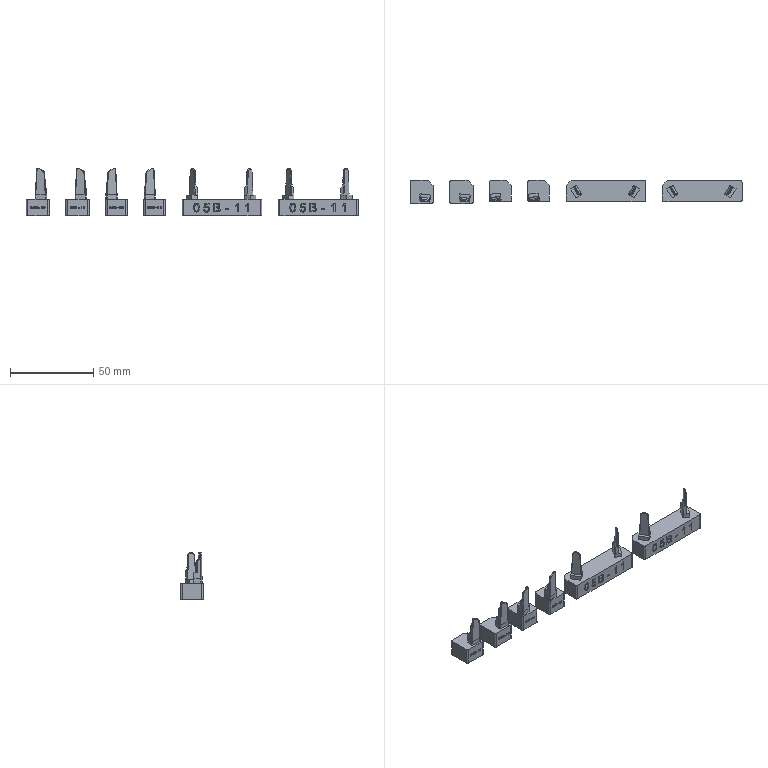NC program | NX | posted with a generic post | part box 200 x 14 x 28.763 mm
Lines 1 to 971 of 209396:
N10 G17 G21 G94 G90
(CAVITY_MILL_C_0_0 , TOOL : D8-0.075)
N12 T00 M6
N14 G53
N16 G17 G0 G90 X0. Y-20.632 S10000 M3
N18 G43 Z30.1 H0
N20 Z0.303
N22 Z-0.197
N24 Y-12.39
N26 G94 G1 X-101.064 F4500.
N28 G2 X-105.391 Y-7.996 R4.39
N30 G1 Y7.992
N32 G2 X-101.065 Y12.388 R4.386
N34 G1 X101.064
N36 G2 X105.391 Y8.077 R4.388
N38 G1 Y-7.992
N40 G2 X101.064 Y-12.39 R4.388
N42 G1 X0.
N44 Y-6.895
N46 X-18.587
N48 G3 X-18.103 Y-3.95 R5.547
N50 G1 X-18.136 Y-3.678
N52 G3 X-22.479 Y1.041 R5.548
N54 X-26.529 Y0.598 R6.416
N56 X-29.797 Y-4.389 R5.567
N58 X-29.293 Y-6.895 R5.637
N60 G1 X-28.292 Y-6.439
N62 G2 X-28.698 Y-4.414 R4.538
N64 X-26.072 Y-0.401 R4.468
N66 X-22.711 Y-0.033 R5.317
N68 X-19.226 Y-3.818 R4.449
N70 G1 X-19.196 Y-4.071
N72 G2 X-21.423 Y-8.426 R4.448
N74 X-25.955 Y-8.728 R5.225
N76 X-28.292 Y-6.439 R4.538
N78 G1 X-29.293 Y-6.895
N80 X-41.584
N82 G3 X-41.105 Y-3.94 R5.551
N84 G1 X-41.135 Y-3.688
N86 G3 X-45.119 Y0.954 R5.558
N88 X-49.527 Y0.603 R6.444
N90 X-52.771 Y-4.882 R5.552
N92 X-52.293 Y-6.895 R5.545
N94 G1 X-51.29 Y-6.446
N96 G2 X-51.674 Y-4.815 R4.446
N98 X-49.071 Y-0.397 R4.453
N100 X-45.422 Y-0.103 R5.345
N102 X-42.226 Y-3.818 R4.459
N104 G1 X-42.196 Y-4.071
N106 G2 X-44.61 Y-8.533 R4.452
N108 X-48.26 Y-8.955 R5.307
N110 X-51.29 Y-6.446 R4.446
N112 G1 X-52.293 Y-6.895
N114 X-63.012
N116 G3 X-62.76 Y-5.757 R5.533
N118 X-65.574 Y-0.105 R5.554
N120 X-70.474 Y0.422 R6.372
N122 X-74.365 Y-4.188 R5.543
N124 G1 X-74.395 Y-4.44
N126 G3 X-74.118 Y-6.895 R5.546
N128 G1 X-73.08 Y-6.531
N130 G2 X-73.304 Y-4.571 R4.447
N132 G1 X-73.274 Y-4.318
N134 G2 X-70.16 Y-0.631 R4.444
N136 X-66.105 Y-1.067 R5.273
N138 X-63.85 Y-5.617 R4.455
N140 X-66.916 Y-9.362 R4.434
N142 X-71.377 Y-8.742 R5.232
N144 X-73.08 Y-6.531 R4.447
N146 G1 X-74.118 Y-6.895
N148 X-87.012
N150 G3 X-86.76 Y-5.757 R5.542
N152 X-89.482 Y-0.152 R5.565
N154 X-94.383 Y0.453 R6.419
N156 X-98.365 Y-4.188 R5.558
N158 G1 X-98.395 Y-4.44
N160 G3 X-98.119 Y-6.895 R5.541
N162 G1 X-97.082 Y-6.531
N164 G2 X-97.304 Y-4.571 R4.442
N166 G1 X-97.274 Y-4.318
N168 G2 X-94.087 Y-0.606 R4.459
N170 X-90.032 Y-1.104 R5.32
N172 X-87.85 Y-5.617 R4.466
N174 X-90.843 Y-9.341 R4.443
N176 X-95.248 Y-8.827 R5.257
N178 X-97.082 Y-6.531 R4.442
N180 G1 X-98.119 Y-6.895
N182 X-99.896
N184 Y6.893
N186 X-77.943
N188 Y1.398
N190 G3 X-79.34 Y-1.4 R11.038
N192 G1 X-81.8
N194 G3 X-83.225 Y1.398 R11.06
N196 G1 X-86.922 Y2.926
N198 X-83.225 Y1.398
N200 X-77.943
N202 X-74.269 Y2.935
N204 X-77.943 Y1.398
N206 Y6.893
N208 X-56.605
N210 Y1.398
N212 G3 X-57.828 Y-1.319 R11.047
N214 X-59.226 Y1.398 R11.049
N216 G1 X-62.925 Y2.925
N218 X-59.226 Y1.398
N220 X-56.605
N222 Y6.893
N224 X-33.606
N226 Y1.398
N228 G3 X-34.857 Y-1.4 R11.062
N230 G1 X-36.007
N232 G3 X-37.232 Y1.398 R11.053
N234 G1 X-33.606
N236 Y6.893
N238 X99.896
N240 Y-6.895
N242 X0.
N244 Y-1.4
N246 X-13.007
N248 G3 X-14.231 Y1.398 R11.043
N250 G1 X94.401
N252 Y-1.4
N254 X0.
N256 Z2.803
N258 G0 Z30.1
N260 Y-20.632
N262 Z0.006
N264 Z-0.494
N266 Y-12.39
N268 G1 X-101.064
N270 G2 X-105.391 Y-7.996 R4.39
N272 G1 Y7.992
N274 G2 X-101.065 Y12.388 R4.386
N276 G1 X101.064
N278 G2 X105.391 Y8.077 R4.388
N280 G1 Y-7.992
N282 G2 X101.064 Y-12.39 R4.388
N284 G1 X0.
N286 Y-6.895
N288 X-18.292
N290 G3 X-17.815 Y-3.908 R5.618
N292 G1 X-17.847 Y-3.642
N294 G3 X-19.013 Y-0.856 R5.512
N296 X-23.738 Y1.279 R5.697
N298 X-24.88 Y1.167 R11.408
N300 X-26.932 Y0.599 R6.733
N302 X-29.794 Y-6.895 R5.693
N304 G1 X-28.789 Y-6.45
N306 G2 X-26.477 Y-0.401 R4.594
N308 X-24.739 Y0.076 R5.634
N310 X-23.685 Y0.181 R10.309
N312 X-19.872 Y-1.542 R4.598
N314 X-18.938 Y-3.772 R4.413
N316 G1 X-18.907 Y-4.038
N318 G2 X-21.074 Y-8.425 R4.519
N320 X-22.85 Y-9.057 R4.782
N322 G1 X-23.116 Y-9.095
N324 G2 X-24.333 Y-9.198 R10.067
N326 X-27.115 Y-8.426 R5.017
N328 X-28.789 Y-6.45 R4.594
N330 G1 X-29.794 Y-6.895
N332 X-41.291
N334 G3 X-40.815 Y-3.908 R5.618
N336 G1 X-40.846 Y-3.651
N338 G3 X-42.925 Y0.058 R5.62
N340 X-46.885 Y1.273 R5.755
N342 X-48.197 Y1.121 R14.817
N344 X-49.935 Y0.598 R6.858
N346 X-52.793 Y-6.895 R5.694
N348 G1 X-51.789 Y-6.45
N350 G2 X-49.482 Y-0.403 R4.595
N352 X-48.023 Y0.036 R5.759
N354 X-46.808 Y0.176 R13.718
N356 X-43.609 Y-0.802 R4.656
N358 X-41.937 Y-3.782 R4.521
N360 G1 X-41.907 Y-4.038
N362 G2 X-44.61 Y-8.702 R4.519
N364 X-46.233 Y-9.108 R5.121
N366 X-47.449 Y-9.2 R8.406
N368 X-50.115 Y-8.426 R5.025
N370 X-51.789 Y-6.45 R4.595
N372 G1 X-52.793 Y-6.895
N374 X-62.514
N376 G3 X-62.951 Y-2.272 R5.744
N378 X-66.544 Y0.459 R5.994
N380 X-67.993 Y0.714 R9.285
N382 X-70.92 Y0.464 R6.098
N384 X-74.654 Y-4.151 R5.602
N386 G1 X-74.685 Y-4.408
N388 G3 X-74.411 Y-6.895 R5.601
N390 G1 X-73.373 Y-6.534
N392 G2 X-73.593 Y-4.538 R4.502
N394 G1 X-73.563 Y-4.282
N396 G2 X-70.566 Y-0.576 R4.503
N398 X-68.132 Y-0.377 R4.999
N400 X-66.831 Y-0.602 R8.186
N402 X-63.91 Y-2.809 R4.895
N404 X-64.744 Y-8.426 R4.645
N406 X-68.132 Y-9.699 R4.948
N408 X-69.349 Y-9.599 R9.552
N410 X-72.105 Y-8.426 R4.809
N412 X-73.373 Y-6.534 R4.502
N414 G1 X-74.411 Y-6.895
N416 X-86.514
N418 G3 X-87.276 Y-1.771 R5.713
N420 X-91.051 Y0.575 R6.069
N422 X-92.353 Y0.756 R17.879
N424 X-94.334 Y0.634 R6.031
N426 X-98.654 Y-4.151 R5.614
N428 G1 X-98.685 Y-4.408
N430 G3 X-98.411 Y-6.895 R5.607
N432 G1 X-97.373 Y-6.534
N434 G2 X-97.593 Y-4.538 R4.508
N436 G1 X-97.563 Y-4.282
N438 G2 X-94.087 Y-0.437 R4.515
N440 X-92.465 Y-0.337 R4.932
N442 X-91.249 Y-0.506 R16.78
N444 X-88.171 Y-2.407 R4.97
N446 X-89.239 Y-8.827 R4.614
N448 X-92.06 Y-9.7 R5.
N450 X-93.276 Y-9.607 R8.43
N452 X-96.115 Y-8.418 R4.867
N454 X-97.373 Y-6.534 R4.508
N456 G1 X-98.411 Y-6.895
N458 X-99.896
N460 Y6.893
N462 X-78.276
N464 Y1.398
N466 G3 X-79.646 Y-1.4 R11.097
N468 G1 X-81.346
N470 G3 X-82.787 Y1.398 R11.208
N472 G1 X-86.501 Y2.918
N474 X-82.787 Y1.398
N476 X-78.276
N478 X-74.632 Y2.947
N480 X-78.276 Y1.398
N482 Y6.893
N484 X-57.039
N486 Y1.398
N488 G3 X-57.86 Y-0.155 R11.189
N490 X-58.157 Y0.413 R11.239
N492 G1 X-58.19 Y0.471
N494 X-58.224 Y0.529
N496 G3 X-58.793 Y1.398 R11.489
N498 G1 X-62.504 Y2.919
N500 X-58.793 Y1.398
N502 X-57.039
N504 Y6.893
N506 X-34.039
N508 Y1.398
N510 G3 X-35.312 Y-1.4 R11.188
N512 G1 X-35.705
N514 G3 X-36.905 Y1.398 R11.115
N516 G1 X-34.039
N518 Y6.893
N520 X-0.953
N522 G3 X-5.721 Y0.969 R5.608
N524 X-5.13 Y-1.277 R6.159
N526 X-3.005 Y-4.222 R11.117
N528 X3.899 Y-4.835 R5.553
N530 X6.261 Y1.057 R5.502
N532 X5.428 Y3.12 R7.766
N534 X3.776 Y5.375 R8.315
N536 X0.701 Y6.893 R5.608
N538 G1 X0.539 Y5.806
N540 G2 X3.011 Y4.585 R4.509
N542 X4.461 Y2.597 R7.216
N544 X5.192 Y0.802 R6.667
N546 X3.312 Y-3.907 R4.403
N548 G1 X3.139 Y-4.016
N550 G2 X-2.231 Y-3.442 R4.454
N552 X-4.139 Y-0.802 R10.018
N554 X-4.625 Y1.043 R5.06
N556 X0.539 Y5.806 R4.509
N558 G1 X0.701 Y6.893
N560 X34.344
N562 G3 X31.79 Y5.848 R5.613
N564 X30.245 Y4.232 R6.854
N566 X28.879 Y1.58 R11.86
N568 X31.274 Y-4.945 R5.541
N570 X38.088 Y-4.142 R5.531
N572 X39.321 Y-2.643 R10.808
N574 X40.559 Y-0.086 R7.654
N576 X38.27 Y5.987 R5.613
N578 X35.914 Y6.893 R5.613
N580 G1 X35.761 Y5.805
N582 G2 X39.498 Y0.201 R4.514
N584 X38.425 Y-2.006 R6.555
N586 X37.311 Y-3.366 R9.709
N588 X31.861 Y-4.016 R4.432
N590 G1 X31.688 Y-3.907
N592 G2 X29.912 Y1.204 R4.442
N594 X31.151 Y3.611 R10.761
N596 X32.444 Y4.964 R5.755
N598 X35.761 Y5.805 R4.514
N600 G1 X35.914 Y6.893
N602 X57.08
N604 G3 X52.383 Y0.173 R5.613
N606 X53.437 Y-2.287 R7.253
N608 G1 X53.668 Y-2.625
N610 G3 X54.989 Y-4.217 R10.717
N612 X61.899 Y-4.835 R5.555
N614 X64.261 Y1.057 R5.504
N616 X63.423 Y3.132 R8.006
N618 X61.736 Y5.41 R8.242
N620 X58.668 Y6.893 R5.613
N622 G1 X58.513 Y5.805
N624 G2 X60.978 Y4.614 R4.514
N626 X62.455 Y2.61 R7.143
N628 X63.192 Y0.802 R6.907
N630 X61.312 Y-3.907 R4.405
N632 G1 X61.139 Y-4.016
N634 G2 X55.763 Y-3.437 R4.456
N636 X54.576 Y-2.006 R9.618
N638 G1 X54.344 Y-1.666
N640 G2 X53.459 Y0.401 R6.154
N642 X58.513 Y5.805 R4.514
N644 G1 X58.668 Y6.893
N646 X92.339
N648 G3 X89.551 Y5.662 R5.613
N650 X88.246 Y4.233 R6.999
N652 X86.88 Y1.579 R11.824
N654 X89.274 Y-4.945 R5.532
N656 X96.14 Y-4.091 R5.534
N658 X97.879 Y-1.767 R12.049
N660 X98.606 Y0.111 R7.004
N662 X96.059 Y6.123 R5.613
N664 X93.916 Y6.893 R5.613
N666 G1 X93.762 Y5.805
N668 G2 X97.535 Y0.357 R4.514
N670 X96.926 Y-1.219 R5.905
N672 X95.353 Y-3.325 R10.95
N674 X89.861 Y-4.016 R4.435
N676 G1 X89.688 Y-3.907
N678 G2 X87.913 Y1.204 R4.433
N680 X89.152 Y3.611 R10.725
N682 X90.252 Y4.815 R5.9
N684 X93.762 Y5.805 R4.514
N686 G1 X93.916 Y6.893
N688 X99.896
N690 Y-6.895
N692 X69.841
N694 Y-1.4
N696 G3 X69.786 Y1.398 R10.999
N698 G1 X81.208
N700 G3 X81.157 Y-1.4 R11.027
N702 G1 X69.841
N704 Y-6.895
N706 X45.895
N708 Y-1.4
N710 G3 X46.237 Y1.398 R11.108
N712 G1 X46.767
N714 G3 X47.014 Y-0.993 R11.108
N716 X47.11 Y-1.4 R12.748
N718 G1 X45.895
N720 Y-6.895
N722 X11.842
N724 Y-1.4
N726 G3 X11.787 Y1.398 R10.997
N728 G1 X23.208
N730 G3 X23.158 Y-1.4 R11.036
N732 G1 X11.842
N734 Y-6.895
N736 X0.
N738 X-10.893 Y-1.4
N740 X-12.701
N742 G3 X-13.901 Y1.398 R11.007
N744 G1 X-11.229
N746 G3 X-11.204 Y0.599 R11.103
N748 X-10.893 Y-1.4 R11.654
N750 G1 Z2.506
N752 G0 X0. Y-20.632
N754 Z-0.29
N756 Z-0.79
N758 Y-12.39
N760 G1 X-101.064
N762 G2 X-105.391 Y-7.996 R4.39
N764 G1 Y7.992
N766 G2 X-101.065 Y12.388 R4.386
N768 G1 X101.064
N770 G2 X105.391 Y8.077 R4.388
N772 G1 Y-7.992
N774 G2 X101.064 Y-12.39 R4.388
N776 G1 X0.
N778 Y-6.895
N780 X-18.153
N782 G3 X-17.677 Y-3.893 R5.641
N784 G1 X-17.708 Y-3.633
N786 G3 X-23.575 Y1.314 R5.634
N788 X-24.13 Y1.264 R7.606
N790 G1 X-25.506 Y1.09
N792 G3 X-27.673 Y0.411 R6.566
N794 X-30.698 Y-5.35 R5.609
N796 X-30.298 Y-6.895 R5.534
N798 G1 X-29.285 Y-6.469
N800 G2 X-29.607 Y-5.216 R4.435
N802 X-27.172 Y-0.568 R4.51
N804 X-25.368 Y0. R5.467
N806 G1 X-23.992 Y0.174
N808 G2 X-23.522 Y0.216 R6.507
N810 X-18.8 Y-3.764 R4.535
N812 G1 X-18.769 Y-4.023
N814 G2 X-22.711 Y-9.051 R4.542
N816 G1 X-24.333 Y-9.235
N818 G2 X-27.172 Y-8.72 R5.18
N820 X-29.285 Y-6.469 R4.435
N822 G1 X-30.298 Y-6.895
N824 X-41.152
N826 G3 X-40.677 Y-3.893 R5.639
N828 G1 X-40.708 Y-3.633
N830 G3 X-46.742 Y1.303 R5.636
N832 X-46.991 Y1.276 R9.11
N834 G1 X-48.499 Y1.091
N836 G3 X-51.165 Y0.125 R6.488
N838 X-53.698 Y-5.352 R5.571
N840 X-53.299 Y-6.895 R5.527
N842 G1 X-52.286 Y-6.469
N844 G2 X-52.607 Y-5.216 R4.428
N846 X-50.575 Y-0.802 R4.472
N848 X-48.365 Y0. R5.389
N850 G1 X-46.856 Y0.185
N852 G2 X-46.638 Y0.209 R8.011
N854 X-41.8 Y-3.764 R4.537
N856 G1 X-41.769 Y-4.023
N858 G2 X-45.422 Y-9.004 R4.54
N860 X-47.449 Y-9.245 R34.868
N862 X-50.288 Y-8.661 R5.185
N864 X-52.286 Y-6.469 R4.428
N866 G1 X-53.299 Y-6.895
N868 X-62.02
N870 G3 X-61.856 Y-6.227 R5.565
N872 X-63.819 Y-0.751 R5.598
N874 X-66.738 Y0.548 R6.312
N876 X-68.838 Y0.809 R39.164
N878 G1 X-68.882 Y0.812
N880 G3 X-74.792 Y-4.133 R5.636
N882 G1 X-74.823 Y-4.393
N884 G3 X-74.55 Y-6.895 R5.638
N886 G1 X-73.511 Y-6.535
N888 G2 X-73.731 Y-4.523 R4.539
N890 G1 X-73.7 Y-4.264
N892 G2 X-68.943 Y-0.285 R4.537
N894 X-66.916 Y-0.536 R38.065
N896 X-64.51 Y-1.605 R5.213
N898 X-62.935 Y-6.019 R4.499
N900 X-65.698 Y-9.39 R4.466
N902 X-68.248 Y-9.725 R5.334
N904 G1 X-69.754 Y-9.555
N906 G2 X-73.511 Y-6.535 R4.539
N908 G1 X-74.55 Y-6.895
N910 X-86.019
N912 G3 X-85.855 Y-6.226 R5.537
N914 X-87.818 Y-0.751 R5.602
N916 X-90.847 Y0.565 R6.297
N918 X-92.757 Y0.804 R47.498
N920 X-98.792 Y-4.133 R5.638
N922 G1 X-98.823 Y-4.393
N924 G3 X-98.548 Y-6.895 R5.641
N926 G1 X-97.51 Y-6.534
N928 G2 X-97.731 Y-4.523 R4.542
N930 G1 X-97.7 Y-4.264
N932 G2 X-92.871 Y-0.29 R4.539
N934 X-91.006 Y-0.523 R46.399
N936 X-88.51 Y-1.605 R5.198
N938 X-86.935 Y-6.019 R4.503
N940 X-89.221 Y-9.165 R4.438
N942 X-92.06 Y-9.744 R5.186
N944 G1 X-93.682 Y-9.563
N946 G2 X-97.51 Y-6.534 R4.542
N948 G1 X-98.548 Y-6.895
N950 X-99.896
N952 Y6.893
N954 X-78.432
N956 Y1.398
N958 G3 X-79.791 Y-1.4 R11.131
N960 G1 X-80.884
N962 G3 X-82.352 Y1.398 R11.097
N964 G1 X-86.084 Y2.911
N966 X-82.352 Y1.398
N968 X-78.432
N970 X-74.8 Y2.953
N972 X-78.432 Y1.398
N974 Y6.893
N976 X-57.493
N978 Y1.398
N980 G3 X-57.896 Y0.718 R11.066
N982 X-58.351 Y1.398 R11.093
N984 G1 X-62.084 Y2.911
N986 X-58.351 Y1.398
N988 X-57.493
N990 Y6.893
N992 X-34.488
N994 Y1.398
N996 G3 X-35.662 Y-1.047 R11.104
N998 X-36.75 Y1.398 R11.131
N1000 G1 X-34.488
N1002 Y6.893
N1004 X-2.496
N1006 G3 X-3.264 Y6.493 R5.575
N1008 G1 X-3.448 Y6.377
N1010 G3 X-5.955 Y2.474 R5.548
N1012 X-5.186 Y-1.363 R6.003
N1014 G1 X-5.001 Y-1.675
N1016 X-4.983 Y-1.704
N1018 X-3.969 Y-3.3
N1020 X-3.951 Y-3.328
N1022 X-3.748 Y-3.627
N1024 G3 X-2.274 Y-5.135 R6.432
N1026 X4.008 Y-5.395 R5.599
N1028 G1 X4.186 Y-5.283
N1030 G3 X6.737 Y-0.351 R5.554
N1032 X5.803 Y2.66 R6.378
N1034 G1 X5.606 Y2.982
N1036 X5.597 Y2.996
N1038 X4.58 Y4.601
N1040 G3 X2.524 Y6.565 R6.177
N1042 X1.874 Y6.893 R5.575
N1044 G1 X1.443 Y5.882
N1046 G2 X1.967 Y5.617 R4.476
N1048 X3.652 Y4.012 R5.078
N1050 G1 X4.669 Y2.407
N1052 X4.867 Y2.085
N1054 G2 X5.639 Y-0.401 R5.279
N1056 X3.598 Y-4.354 R4.455
N1058 G1 X3.42 Y-4.467
N1060 G2 X-1.622 Y-4.25 R4.5
N1062 X-2.839 Y-3.009 R5.333
N1064 G1 X-3.042 Y-2.711
N1066 X-4.055 Y-1.114
N1068 X-4.241 Y-0.802
N1070 G2 X-4.867 Y2.321 R4.904
N1072 X-2.86 Y5.448 R4.449
N1074 G1 X-2.676 Y5.564
N1076 G2 X1.443 Y5.882 R4.476
N1078 G1 X1.874 Y6.893
N1080 X33.121
N1082 G3 X32.469 Y6.564 R5.587
N1084 X30.425 Y4.61 R6.272
N1086 G1 X30.305 Y4.425
N1088 X30.298 Y4.414
N1090 X29.284 Y2.806
N1092 X29.269 Y2.782
N1094 X29.142 Y2.568
N1096 G3 X28.264 Y-0.345 R6.367
N1098 X30.814 Y-5.283 R5.565
N1100 G1 X30.992 Y-5.395
N1102 G3 X37.125 Y-5.241 R5.597
N1104 X38.904 Y-3.399 R6.746
N1106 G1 X39.926 Y-1.794
N1108 X39.939 Y-1.773
N1110 X40.107 Y-1.495
N1112 G3 X40.918 Y0.621 R6.368
N1114 X38.448 Y6.377 R5.607
N1116 G1 X38.264 Y6.493
N1118 G3 X37.494 Y6.893 R5.587
N1120 G1 X37.064 Y5.882
N1122 G2 X37.676 Y5.564 R4.488
N1124 G1 X37.86 Y5.448
N1126 G2 X39.839 Y0.825 R4.508
N1128 X39.168 Y-0.925 R5.269
N1130 G1 X38.999 Y-1.204
N1132 X37.977 Y-2.809
N1134 G2 X36.499 Y-4.337 R5.647
N1136 X31.58 Y-4.467 R4.498
N1138 G1 X31.402 Y-4.354
N1140 G2 X29.361 Y-0.401 R4.466
N1142 X30.086 Y2.006 R5.268
N1144 G1 X30.213 Y2.22
N1146 X31.227 Y3.827
N1148 X31.347 Y4.012
N1150 G2 X33.027 Y5.617 R5.173
N1152 X37.064 Y5.882 R4.488
N1154 G1 X37.494 Y6.893
N1156 X55.508
N1158 G3 X54.736 Y6.493 R5.61
N1160 G1 X54.552 Y6.377
N1162 G3 X52.037 Y2.408 R5.546
N1164 X52.814 Y-1.356 R5.967
N1166 G1 X52.987 Y-1.654
N1168 X53.011 Y-1.694
N1170 X54.096 Y-3.399
N1172 X54.123 Y-3.44
N1174 X54.253 Y-3.624
N1176 G3 X55.718 Y-5.13 R6.357
N1178 X62.008 Y-5.395 R5.597
N1180 G1 X62.186 Y-5.283
N1182 G3 X64.737 Y-0.351 R5.557
N1184 X63.862 Y2.561 R6.382
N1186 G1 X63.81 Y2.65
N1188 X63.789 Y2.685
N1190 X62.629 Y4.521
N1192 G3 X61.223 Y6.089 R6.327
N1194 G1 X61.112 Y6.178
N1196 G3 X59.885 Y6.893 R5.61
N1198 G1 X59.457 Y5.881
N1200 G2 X60.427 Y5.319 R4.511
N1202 G1 X60.538 Y5.23
N1204 G2 X61.7 Y3.934 R5.228
N1206 G1 X62.86 Y2.098
N1208 X62.913 Y2.006
N1210 G2 X63.639 Y-0.401 R5.283
N1212 X61.598 Y-4.354 R4.458
N1214 G1 X61.42 Y-4.467
N1216 G2 X56.371 Y-4.246 R4.498
N1218 X55.155 Y-2.996 R5.258
N1220 G1 X55.023 Y-2.809
N1222 X53.938 Y-1.104
N1224 X53.764 Y-0.802
N1226 G2 X53.127 Y2.268 R4.868
N1228 X55.14 Y5.448 R4.447
N1230 G1 X55.324 Y5.564
N1232 G2 X59.457 Y5.881 R4.511
N1234 G1 X59.885 Y6.893
N1236 X91.121
N1238 G3 X90.468 Y6.564 R5.589
N1240 X88.419 Y4.6 R6.285
N1242 G1 X87.402 Y2.995
N1244 X87.389 Y2.974
N1246 X87.148 Y2.573
N1248 G3 X86.264 Y-0.347 R6.293
N1250 X88.807 Y-5.278 R5.563
N1252 G1 X89.003 Y-5.402
N1254 G3 X95.117 Y-5.246 R5.596
N1256 X96.904 Y-3.399 R6.706
N1258 G1 X97.926 Y-1.794
N1260 X97.937 Y-1.776
N1262 X98.182 Y-1.374
N1264 G3 X99.012 Y1.582 R6.14
N1266 X96.448 Y6.377 R5.58
N1268 G1 X96.264 Y6.493
N1270 G3 X95.494 Y6.893 R5.589
N1272 G1 X95.064 Y5.882
N1274 G2 X95.676 Y5.564 R4.49
N1276 G1 X95.86 Y5.448
N1278 G2 X97.913 Y1.605 R4.481
N1280 X97.243 Y-0.802 R5.041
N1282 G1 X96.999 Y-1.204
N1284 X95.977 Y-2.809
N1286 G2 X94.493 Y-4.341 R5.607
N1288 X89.58 Y-4.467 R4.497
N1290 G1 X89.402 Y-4.354
N1292 G2 X87.361 Y-0.401 R4.464
N1294 X88.089 Y2.006 R5.194
N1296 G1 X88.331 Y2.407
N1298 X89.347 Y4.012
N1300 G2 X91.027 Y5.617 R5.186
N1302 X95.064 Y5.882 R4.49
N1304 G1 X95.494 Y6.893
N1306 X99.896
N1308 Y-6.895
N1310 X70.209
N1312 Y-1.4
N1314 G3 X70.226 Y-0.085 R11.052
N1316 X70.058 Y1.398 R11.877
N1318 G1 X80.941
N1320 G3 X80.775 Y-0.086 R11.788
N1322 X80.792 Y-1.4 R11.058
N1324 G1 X70.209
N1326 Y-6.895
N1328 X46.083
N1330 Y-1.4
N1332 G3 X46.317 Y-0.402 R11.863
N1334 X46.504 Y1.249 R11.102
N1336 X46.914 Y-1.4 R11.462
N1338 G1 X46.083
N1340 Y-6.895
N1342 X12.209
N1344 Y-1.4
N1346 G3 X12.225 Y-0.084 R11.049
N1348 X12.058 Y1.398 R11.873
N1350 G1 X22.943
N1352 G3 X22.775 Y-0.076 R11.862
N1354 X22.792 Y-1.4 R11.06
N1356 G1 X12.209
N1358 Y-6.895
N1360 X0.
N1362 X-11.086 Y-1.4
N1364 X-12.56
N1366 G3 X-13.75 Y1.398 R11.129
N1368 G1 X-11.501
N1370 G3 X-11.086 Y-1.4 R11.498
N1372 G1 Z2.21
N1374 G0 X0. Y-20.632
N1376 Z-0.587
N1378 Z-1.087
N1380 Y-12.39
N1382 G1 X-101.064
N1384 G2 X-105.391 Y-7.996 R4.39
N1386 G1 Y7.992
N1388 G2 X-101.065 Y12.388 R4.386
N1390 G1 X101.064
N1392 G2 X105.391 Y8.077 R4.388
N1394 G1 Y-7.992
N1396 G2 X101.064 Y-12.39 R4.388
N1398 G1 X0.
N1400 Y-6.895
N1402 X-18.103
N1404 G3 X-17.631 Y-3.891 R5.632
N1406 G1 X-17.663 Y-3.626
N1408 G3 X-23.953 Y1.288 R5.625
N1410 G1 X-26.093 Y1.018
N1412 G3 X-30.145 Y-1.339 R6.14
N1414 X-30.797 Y-6.895 R5.725
N1416 G1 X-29.782 Y-6.473
N1418 G2 X-29.271 Y-2.006 R4.626
N1420 X-25.955 Y-0.073 R5.041
N1422 G1 X-23.815 Y0.197
N1424 G2 X-18.754 Y-3.757 R4.526
N1426 G1 X-18.722 Y-4.019
N1428 G2 X-22.711 Y-9.054 R4.533
N1430 G1 X-24.739 Y-9.285
N1432 G2 X-26.361 Y-9.219 R5.737
N1434 X-28.794 Y-7.957 R4.775
N1436 X-29.782 Y-6.473 R4.626
N1438 G1 X-30.797 Y-6.895
N1440 X-41.103
N1442 G3 X-40.631 Y-3.89 R5.63
N1444 G1 X-40.663 Y-3.624
N1446 G3 X-46.893 Y1.293 R5.621
N1448 G1 X-47.171 Y1.26
N1450 X-47.18 Y1.259
N1452 X-48.933 Y1.04
N1454 G3 X-51.118 Y0.372 R6.666
N1456 X-53.795 Y-6.895 R5.687
N1458 G1 X-52.781 Y-6.471
N1460 G2 X-50.621 Y-0.608 R4.588
N1462 X-48.796 Y-0.051 R5.567
N1464 G1 X-47.044 Y0.169
N1466 X-46.766 Y0.201
N1468 G2 X-41.754 Y-3.754 R4.522
N1470 G1 X-41.722 Y-4.019
N1472 G2 X-45.422 Y-9.012 R4.531
N1474 G1 X-45.827 Y-9.067
N1476 X-47.449 Y-9.252
N1478 X-47.759 Y-9.286
N1480 G2 X-50.555 Y-8.827 R5.292
N1482 X-52.781 Y-6.471 R4.588
N1484 G1 X-53.795 Y-6.895
N1486 X-61.521
N1488 G3 X-62.865 Y-1.242 R5.692
N1490 X-66.328 Y0.505 R6.216
N1492 G1 X-66.372 Y0.511
N1494 X-68.399 Y0.769
N1496 X-68.826 Y0.815
N1498 X-68.869 Y0.819
N1500 G3 X-74.837 Y-4.125 R5.629
N1502 G1 X-74.869 Y-4.389
N1504 G3 X-74.597 Y-6.895 R5.631
N1506 G1 X-73.559 Y-6.535
N1508 G2 X-73.778 Y-4.519 R4.532
N1510 G1 X-73.746 Y-4.256
N1512 G2 X-68.943 Y-0.278 R4.53
N1514 G1 X-68.538 Y-0.321
N1516 X-66.51 Y-0.579
N1518 X-66.376 Y-0.602
N1520 G2 X-63.655 Y-2.006 R5.117
N1522 X-66.079 Y-9.708 R4.593
N1524 X-67.831 Y-9.777 R5.764
N1526 G1 X-69.754 Y-9.558
N1528 G2 X-73.559 Y-6.535 R4.532
N1530 G1 X-74.597 Y-6.895
N1532 X-85.521
N1534 G3 X-86.865 Y-1.242 R5.691
N1536 X-90.235 Y0.49 R6.22
N1538 G1 X-90.298 Y0.5
N1540 X-92.326 Y0.76
N1542 X-92.78 Y0.811
N1544 G3 X-98.837 Y-4.125 R5.631
N1546 G1 X-98.869 Y-4.389
N1548 G3 X-98.597 Y-6.895 R5.634
N1550 G1 X-97.558 Y-6.535
N1552 G2 X-97.778 Y-4.519 R4.535
N1554 G1 X-97.746 Y-4.256
N1556 G2 X-92.871 Y-0.284 R4.532
N1558 G1 X-92.465 Y-0.33
N1560 X-90.438 Y-0.59
N1562 X-90.373 Y-0.602
N1564 G2 X-87.655 Y-2.006 R5.121
N1566 X-90.035 Y-9.699 R4.592
N1568 X-91.792 Y-9.781 R5.696
N1570 G1 X-92.06 Y-9.751
N1572 X-93.682 Y-9.566
N1574 X-94.087 Y-9.51
N1576 G2 X-97.558 Y-6.535 R4.535
N1578 G1 X-98.597 Y-6.895
N1580 X-99.896
N1582 Y6.893
N1584 X-78.487
N1586 Y1.398
N1588 G3 X-79.841 Y-1.4 R11.124
N1590 G1 X-80.433
N1592 G3 X-81.921 Y1.398 R11.186
N1594 G1 X-85.671 Y2.904
N1596 X-81.921 Y1.398
N1598 X-78.487
N1600 X-74.859 Y2.954
N1602 X-78.487 Y1.398
N1604 Y6.893
N1606 X-57.922
N1608 X-57.92 Y1.398
N1610 X-57.921 Y1.397
N1612 X-57.922 Y1.398
N1614 X-61.671 Y2.904
N1616 X-57.922 Y1.398
N1618 X-57.92
N1620 X-57.922 Y6.893
N1622 X-34.928
N1624 Y1.398
N1626 G3 X-35.851 Y-0.347 R11.22
N1628 X-36.694 Y1.398 R11.116
N1630 G1 X-34.928
N1632 X-31.329 Y2.968
N1634 X-34.928 Y1.398
N1636 Y6.893
N1638 X-3.129
N1640 G3 X-3.411 Y6.728 R5.604
N1642 G1 X-3.597 Y6.61
N1644 G3 X-5.912 Y3.611 R5.618
N1646 X-5.331 Y-1.151 R5.801
N1648 G1 X-5.195 Y-1.375
N1650 X-5.184 Y-1.391
N1652 X-3.692 Y-3.742
N1654 G3 X-2.342 Y-5.259 R6.292
N1656 X4.175 Y-5.662 R5.623
N1658 G1 X4.355 Y-5.547
N1660 G3 X6.853 Y-1.795 R5.605
N1662 X6.047 Y2.284 R5.905
N1664 G1 X5.86 Y2.585
N1666 X5.855 Y2.593
N1668 X4.376 Y4.933
N1670 X4.358 Y4.96
N1672 G3 X2.727 Y6.61 R5.902
N1674 G1 X2.626 Y6.675
N1676 G3 X2.262 Y6.893 R5.604
N1678 G1 X1.734 Y5.93
N1680 G2 X2.028 Y5.754 R4.505
N1682 G1 X2.113 Y5.699
N1684 G2 X3.401 Y4.414 R4.803
N1686 G1 X3.447 Y4.346
N1688 X4.926 Y2.006
N1690 X5.113 Y1.705
N1692 G2 X5.771 Y-1.605 R4.806
N1694 X3.767 Y-4.619 R4.506
N1696 G1 X3.587 Y-4.733
N1698 G2 X-1.65 Y-4.405 R4.524
N1700 X-2.765 Y-3.153 R5.193
N1702 G1 X-4.256 Y-0.802
N1704 X-4.393 Y-0.579
N1706 G2 X-4.867 Y3.272 R4.702
N1708 X-3.01 Y5.681 R4.519
N1710 G1 X-2.823 Y5.799
N1712 G2 X1.734 Y5.93 R4.505
N1714 G1 X2.262 Y6.893
N1716 X32.742
N1718 G3 X30.676 Y5.009 R5.824
N1720 G1 X30.418 Y4.608
N1722 X30.412 Y4.599
N1724 X29.013 Y2.384
N1726 G3 X28.353 Y0.987 R6.378
N1728 X29.115 Y-4.099 R5.689
N1730 X31.849 Y-6.166 R6.073
N1732 X35.092 Y-6.363 R5.486
N1734 X38.547 Y-3.961 R5.858
N1736 G1 X38.639 Y-3.826
N1738 X38.656 Y-3.799
N1740 X40.266 Y-1.262
N1742 G3 X41.012 Y0.481 R6.02
N1744 X38.259 Y6.815 R5.642
N1746 G1 X38.122 Y6.893
N1748 X37.592 Y5.931
N1750 X37.716 Y5.86
N1752 G2 X39.947 Y0.75 R4.543
N1754 X39.338 Y-0.673 R4.921
N1756 G1 X37.728 Y-3.21
N1758 X37.638 Y-3.344
N1760 G2 X34.83 Y-5.295 R4.759
N1762 X32.237 Y-5.138 R4.387
N1764 X30.011 Y-3.463 R4.974
N1766 X29.396 Y0.641 R4.59
N1768 X29.943 Y1.798 R5.279
N1770 G1 X31.341 Y4.012
N1772 X31.6 Y4.414
N1774 G2 X34.066 Y6.27 R4.725
N1776 X37.592 Y5.931 R4.47
N1778 G1 X38.122 Y6.893
N1780 X54.869
N1782 G3 X54.589 Y6.728 R5.552
N1784 G1 X54.403 Y6.61
N1786 G3 X52.08 Y3.587 R5.618
N1788 X52.664 Y-1.143 R5.784
N1790 G1 X52.805 Y-1.375
N1792 X52.816 Y-1.391
N1794 X54.344 Y-3.799
N1796 X54.362 Y-3.827
N1798 X54.439 Y-3.94
N1800 G3 X56.168 Y-5.626 R6.005
N1802 X62.175 Y-5.662 R5.617
N1804 G1 X62.355 Y-5.547
N1806 G3 X64.854 Y-1.795 R5.61
N1808 X64.048 Y2.281 R5.898
N1810 G1 X63.859 Y2.585
N1812 X63.854 Y2.593
N1814 X62.37 Y4.942
N1816 G3 X60.258 Y6.893 R5.858
N1818 G1 X59.733 Y5.928
N1820 G2 X61.401 Y4.414 R4.759
N1822 G1 X61.441 Y4.355
N1824 X62.925 Y2.006
N1826 X63.114 Y1.702
N1828 G2 X63.771 Y-1.605 R4.799
N1830 X61.767 Y-4.619 R4.511
N1832 G1 X61.587 Y-4.733
N1834 G2 X56.761 Y-4.7 R4.518
N1836 X55.348 Y-3.323 R4.906
N1838 G1 X55.272 Y-3.21
N1840 X53.744 Y-0.802
N1842 X53.602 Y-0.571
N1844 G2 X53.127 Y3.253 R4.685
N1846 X54.99 Y5.681 R4.519
N1848 G1 X55.177 Y5.799
N1850 G2 X59.017 Y6.244 R4.453
N1852 X59.733 Y5.928 R4.759
N1854 G1 X60.258 Y6.893
N1856 X90.739
N1858 G3 X88.674 Y5.008 R5.907
N1860 G1 X88.416 Y4.606
N1862 X88.412 Y4.599
N1864 X87.012 Y2.382
N1866 G3 X86.349 Y0.977 R6.349
N1868 X87.106 Y-4.088 R5.695
N1870 X90.124 Y-6.262 R6.056
N1872 X94.14 Y-6.001 R5.638
N1874 X96.656 Y-3.799 R5.976
N1876 G1 X98.26 Y-1.273
N1878 G3 X99.122 Y1.04 R5.992
N1880 X96.25 Y6.819 R5.633
N1882 G1 X96.12 Y6.893
N1884 X95.591 Y5.93
N1886 X95.71 Y5.863
N1888 G2 X98.036 Y1.204 R4.534
N1890 X97.332 Y-0.684 R4.893
N1892 G1 X95.728 Y-3.21
N1894 X95.691 Y-3.267
N1896 G2 X93.682 Y-5.002 R4.877
N1898 X90.461 Y-5.216 R4.539
N1900 X88.004 Y-3.454 R4.957
N1902 X87.393 Y0.633 R4.596
N1904 X87.941 Y1.795 R5.25
N1906 G1 X89.341 Y4.012
N1908 X89.599 Y4.414
N1910 G2 X91.654 Y6.119 R4.808
N1912 X95.591 Y5.93 R4.49
N1914 G1 X96.12 Y6.893
N1916 X99.896
N1918 Y-6.895
N1920 X70.414
N1922 Y-1.4
N1924 G3 X70.209 Y1.398 R11.393
N1926 G1 X80.788
N1928 G3 X80.585 Y-1.4 R11.19
N1930 G1 X70.414
N1932 Y-6.895
N1934 X46.191
N1936 Y-1.4
N1938 G3 X46.34 Y-0.864 R11.515
N1940 X46.501 Y-0.124 R11.137